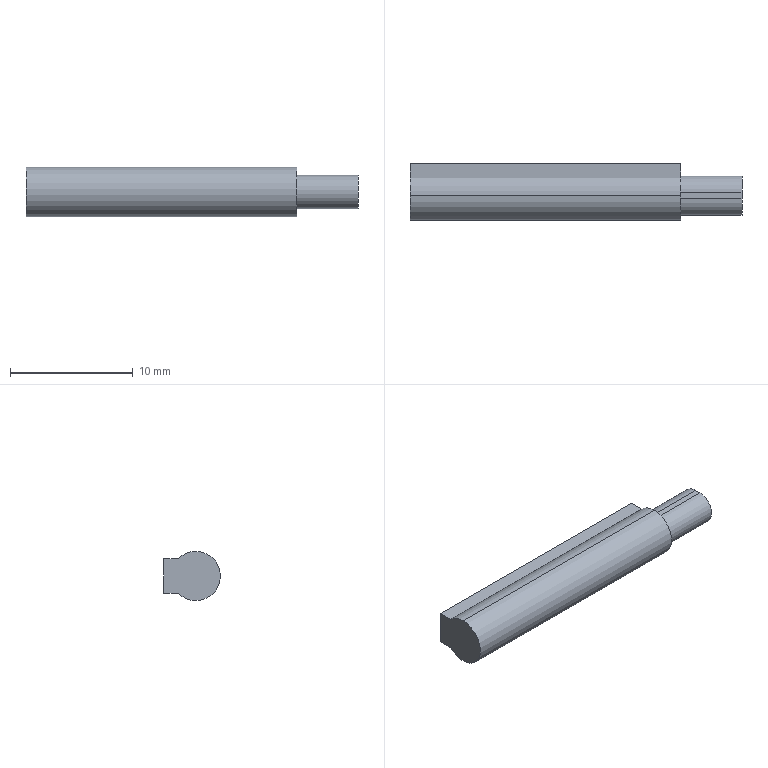Part | SolidWorks | features BaseBody 1 | 1 solid | 16 faces | box 27 x 4.6 x 4 mm | volume 359.458 mm3 | plane 9 | cylinder 7 | commonest cylinder face diameters 4 x3 2 x2 2.7 x2
STEP:
#1=CARTESIAN_POINT('',(22.,1.428,-1.4));
#2=VERTEX_POINT('',#1);
#3=CARTESIAN_POINT('',(22.,0.,-2.));
#4=VERTEX_POINT('',#3);
#5=CARTESIAN_POINT('',(22.,0.,0.));
#6=DIRECTION('',(-1.,0.,0.));
#7=DIRECTION('',(0.,0.,1.));
#8=AXIS2_PLACEMENT_3D('',#5,#6,#7);
#9=CIRCLE('',#8,2.);
#10=EDGE_CURVE('',#2,#4,#9,.T.);
#11=ORIENTED_EDGE('',*,*,#10,.T.);
#12=CARTESIAN_POINT('',(0.,0.,-2.));
#13=VERTEX_POINT('',#12);
#14=CARTESIAN_POINT('',(22.,0.,-2.));
#15=DIRECTION('',(-1.,0.,0.));
#16=VECTOR('',#15,1000.);
#17=LINE('',#14,#16);
#18=EDGE_CURVE('',#4,#13,#17,.T.);
#19=ORIENTED_EDGE('',*,*,#18,.T.);
#20=CARTESIAN_POINT('',(0.,1.428,-1.4));
#21=VERTEX_POINT('',#20);
#22=CARTESIAN_POINT('',(0.,0.,0.));
#23=DIRECTION('',(1.,0.,0.));
#24=DIRECTION('',(0.,0.,1.));
#25=AXIS2_PLACEMENT_3D('',#22,#23,#24);
#26=CIRCLE('',#25,2.);
#27=EDGE_CURVE('',#13,#21,#26,.T.);
#28=ORIENTED_EDGE('',*,*,#27,.T.);
#29=CARTESIAN_POINT('',(22.,1.428,-1.4));
#30=DIRECTION('',(1.,0.,0.));
#31=VECTOR('',#30,1000.);
#32=LINE('',#29,#31);
#33=EDGE_CURVE('',#21,#2,#32,.T.);
#34=ORIENTED_EDGE('',*,*,#33,.T.);
#35=EDGE_LOOP('',(#11,#19,#28,#34));
#36=FACE_OUTER_BOUND('',#35,.T.);
#37=CARTESIAN_POINT('',(22.,0.,0.));
#38=DIRECTION('',(-1.,0.,0.));
#39=DIRECTION('',(0.,0.,1.));
#40=AXIS2_PLACEMENT_3D('',#37,#38,#39);
#41=CYLINDRICAL_SURFACE('',#40,2.);
#42=ADVANCED_FACE('',(#36),#41,.T.);
#43=ORIENTED_EDGE('',*,*,#18,.F.);
#44=CARTESIAN_POINT('',(22.,0.,2.));
#45=VERTEX_POINT('',#44);
#46=CARTESIAN_POINT('',(22.,0.,0.));
#47=DIRECTION('',(-1.,0.,0.));
#48=DIRECTION('',(0.,0.,1.));
#49=AXIS2_PLACEMENT_3D('',#46,#47,#48);
#50=CIRCLE('',#49,2.);
#51=EDGE_CURVE('',#4,#45,#50,.T.);
#52=ORIENTED_EDGE('',*,*,#51,.T.);
#53=CARTESIAN_POINT('',(0.,0.,2.));
#54=VERTEX_POINT('',#53);
#55=CARTESIAN_POINT('',(22.,0.,2.));
#56=DIRECTION('',(-1.,0.,0.));
#57=VECTOR('',#56,1000.);
#58=LINE('',#55,#57);
#59=EDGE_CURVE('',#45,#54,#58,.T.);
#60=ORIENTED_EDGE('',*,*,#59,.T.);
#61=CARTESIAN_POINT('',(0.,0.,0.));
#62=DIRECTION('',(1.,0.,0.));
#63=DIRECTION('',(0.,0.,1.));
#64=AXIS2_PLACEMENT_3D('',#61,#62,#63);
#65=CIRCLE('',#64,2.);
#66=EDGE_CURVE('',#54,#13,#65,.T.);
#67=ORIENTED_EDGE('',*,*,#66,.T.);
#68=EDGE_LOOP('',(#43,#52,#60,#67));
#69=FACE_OUTER_BOUND('',#68,.T.);
#70=CARTESIAN_POINT('',(22.,0.,0.));
#71=DIRECTION('',(-1.,0.,0.));
#72=DIRECTION('',(0.,0.,1.));
#73=AXIS2_PLACEMENT_3D('',#70,#71,#72);
#74=CYLINDRICAL_SURFACE('',#73,2.);
#75=ADVANCED_FACE('',(#69),#74,.T.);
#76=CARTESIAN_POINT('',(2.,2.5,-1.));
#77=VERTEX_POINT('',#76);
#78=CARTESIAN_POINT('',(2.,2.5,1.));
#79=VERTEX_POINT('',#78);
#80=CARTESIAN_POINT('',(2.,2.5,0.));
#81=DIRECTION('',(0.,1.,0.));
#82=DIRECTION('',(0.,0.,1.));
#83=AXIS2_PLACEMENT_3D('',#80,#81,#82);
#84=CIRCLE('',#83,1.);
#85=EDGE_CURVE('',#77,#79,#84,.T.);
#86=ORIENTED_EDGE('',*,*,#85,.F.);
#87=CARTESIAN_POINT('',(2.,2.6,-1.));
#88=VERTEX_POINT('',#87);
#89=CARTESIAN_POINT('',(2.,2.6,-1.));
#90=DIRECTION('',(0.,1.,0.));
#91=VECTOR('',#90,1000.);
#92=LINE('',#89,#91);
#93=EDGE_CURVE('',#77,#88,#92,.T.);
#94=ORIENTED_EDGE('',*,*,#93,.T.);
#95=CARTESIAN_POINT('',(2.,2.6,1.));
#96=VERTEX_POINT('',#95);
#97=CARTESIAN_POINT('',(2.,2.6,0.));
#98=DIRECTION('',(0.,1.,0.));
#99=DIRECTION('',(0.,0.,1.));
#100=AXIS2_PLACEMENT_3D('',#97,#98,#99);
#101=CIRCLE('',#100,1.);
#102=EDGE_CURVE('',#88,#96,#101,.T.);
#103=ORIENTED_EDGE('',*,*,#102,.T.);
#104=CARTESIAN_POINT('',(2.,2.6,1.));
#105=DIRECTION('',(0.,1.,0.));
#106=VECTOR('',#105,1000.);
#107=LINE('',#104,#106);
#108=EDGE_CURVE('',#79,#96,#107,.T.);
#109=ORIENTED_EDGE('',*,*,#108,.F.);
#110=EDGE_LOOP('',(#86,#94,#103,#109));
#111=FACE_OUTER_BOUND('',#110,.T.);
#112=CARTESIAN_POINT('',(2.,2.6,0.));
#113=DIRECTION('',(0.,1.,0.));
#114=DIRECTION('',(0.,0.,1.));
#115=AXIS2_PLACEMENT_3D('',#112,#113,#114);
#116=CYLINDRICAL_SURFACE('',#115,1.);
#117=ADVANCED_FACE('',(#111),#116,.F.);
#118=ORIENTED_EDGE('',*,*,#59,.F.);
#119=CARTESIAN_POINT('',(22.,1.428,1.4));
#120=VERTEX_POINT('',#119);
#121=CARTESIAN_POINT('',(22.,0.,0.));
#122=DIRECTION('',(-1.,0.,0.));
#123=DIRECTION('',(0.,0.,1.));
#124=AXIS2_PLACEMENT_3D('',#121,#122,#123);
#125=CIRCLE('',#124,2.);
#126=EDGE_CURVE('',#45,#120,#125,.T.);
#127=ORIENTED_EDGE('',*,*,#126,.T.);
#128=CARTESIAN_POINT('',(0.,1.428,1.4));
#129=VERTEX_POINT('',#128);
#130=CARTESIAN_POINT('',(22.,1.428,1.4));
#131=DIRECTION('',(-1.,0.,0.));
#132=VECTOR('',#131,1000.);
#133=LINE('',#130,#132);
#134=EDGE_CURVE('',#120,#129,#133,.T.);
#135=ORIENTED_EDGE('',*,*,#134,.T.);
#136=CARTESIAN_POINT('',(0.,0.,0.));
#137=DIRECTION('',(1.,0.,0.));
#138=DIRECTION('',(0.,0.,1.));
#139=AXIS2_PLACEMENT_3D('',#136,#137,#138);
#140=CIRCLE('',#139,2.);
#141=EDGE_CURVE('',#129,#54,#140,.T.);
#142=ORIENTED_EDGE('',*,*,#141,.T.);
#143=EDGE_LOOP('',(#118,#127,#135,#142));
#144=FACE_OUTER_BOUND('',#143,.T.);
#145=CARTESIAN_POINT('',(22.,0.,0.));
#146=DIRECTION('',(-1.,0.,0.));
#147=DIRECTION('',(0.,0.,1.));
#148=AXIS2_PLACEMENT_3D('',#145,#146,#147);
#149=CYLINDRICAL_SURFACE('',#148,2.);
#150=ADVANCED_FACE('',(#144),#149,.T.);
#151=CARTESIAN_POINT('',(0.,2.6,1.4));
#152=VERTEX_POINT('',#151);
#153=CARTESIAN_POINT('',(0.,2.6,1.4));
#154=DIRECTION('',(0.,1.,0.));
#155=VECTOR('',#154,1000.);
#156=LINE('',#153,#155);
#157=EDGE_CURVE('',#129,#152,#156,.T.);
#158=ORIENTED_EDGE('',*,*,#157,.T.);
#159=CARTESIAN_POINT('',(0.,2.6,-1.4));
#160=VERTEX_POINT('',#159);
#161=CARTESIAN_POINT('',(0.,2.6,0.));
#162=DIRECTION('',(0.,0.,1.));
#163=VECTOR('',#162,1000.);
#164=LINE('',#161,#163);
#165=EDGE_CURVE('',#160,#152,#164,.T.);
#166=ORIENTED_EDGE('',*,*,#165,.F.);
#167=CARTESIAN_POINT('',(0.,1.428,-1.4));
#168=DIRECTION('',(0.,-1.,0.));
#169=VECTOR('',#168,1000.);
#170=LINE('',#167,#169);
#171=EDGE_CURVE('',#160,#21,#170,.T.);
#172=ORIENTED_EDGE('',*,*,#171,.T.);
#173=ORIENTED_EDGE('',*,*,#27,.F.);
#174=ORIENTED_EDGE('',*,*,#66,.F.);
#175=ORIENTED_EDGE('',*,*,#141,.F.);
#176=EDGE_LOOP('',(#158,#166,#172,#173,#174,#175));
#177=FACE_OUTER_BOUND('',#176,.T.);
#178=CARTESIAN_POINT('',(0.,0.,0.));
#179=DIRECTION('',(1.,0.,0.));
#180=DIRECTION('',(0.,0.,-1.));
#181=AXIS2_PLACEMENT_3D('',#178,#179,#180);
#182=PLANE('',#181);
#183=ADVANCED_FACE('',(#177),#182,.F.);
#184=CARTESIAN_POINT('',(22.,-0.25,1.35));
#185=VERTEX_POINT('',#184);
#186=CARTESIAN_POINT('',(22.,0.25,1.35));
#187=VERTEX_POINT('',#186);
#188=CARTESIAN_POINT('',(22.,0.25,1.35));
#189=DIRECTION('',(0.,1.,0.));
#190=VECTOR('',#189,1000.);
#191=LINE('',#188,#190);
#192=EDGE_CURVE('',#185,#187,#191,.T.);
#193=ORIENTED_EDGE('',*,*,#192,.T.);
#194=CARTESIAN_POINT('',(22.,0.25,-1.35));
#195=VERTEX_POINT('',#194);
#196=CARTESIAN_POINT('',(22.,0.25,0.));
#197=DIRECTION('',(-1.,0.,0.));
#198=DIRECTION('',(0.,0.,1.));
#199=AXIS2_PLACEMENT_3D('',#196,#197,#198);
#200=CIRCLE('',#199,1.35);
#201=EDGE_CURVE('',#187,#195,#200,.T.);
#202=ORIENTED_EDGE('',*,*,#201,.T.);
#203=CARTESIAN_POINT('',(22.,-0.25,-1.35));
#204=VERTEX_POINT('',#203);
#205=CARTESIAN_POINT('',(22.,-0.25,-1.35));
#206=DIRECTION('',(0.,-1.,0.));
#207=VECTOR('',#206,1000.);
#208=LINE('',#205,#207);
#209=EDGE_CURVE('',#195,#204,#208,.T.);
#210=ORIENTED_EDGE('',*,*,#209,.T.);
#211=CARTESIAN_POINT('',(22.,-0.25,0.));
#212=DIRECTION('',(-1.,0.,0.));
#213=DIRECTION('',(0.,0.,1.));
#214=AXIS2_PLACEMENT_3D('',#211,#212,#213);
#215=CIRCLE('',#214,1.35);
#216=EDGE_CURVE('',#204,#185,#215,.T.);
#217=ORIENTED_EDGE('',*,*,#216,.T.);
#218=EDGE_LOOP('',(#193,#202,#210,#217));
#219=FACE_BOUND('',#218,.T.);
#220=CARTESIAN_POINT('',(22.,2.6,-1.4));
#221=VERTEX_POINT('',#220);
#222=CARTESIAN_POINT('',(22.,2.6,1.4));
#223=VERTEX_POINT('',#222);
#224=CARTESIAN_POINT('',(22.,2.6,0.));
#225=DIRECTION('',(0.,0.,1.));
#226=VECTOR('',#225,1000.);
#227=LINE('',#224,#226);
#228=EDGE_CURVE('',#221,#223,#227,.T.);
#229=ORIENTED_EDGE('',*,*,#228,.T.);
#230=CARTESIAN_POINT('',(22.,0.,1.4));
#231=DIRECTION('',(0.,-1.,0.));
#232=VECTOR('',#231,1000.);
#233=LINE('',#230,#232);
#234=EDGE_CURVE('',#223,#120,#233,.T.);
#235=ORIENTED_EDGE('',*,*,#234,.T.);
#236=ORIENTED_EDGE('',*,*,#126,.F.);
#237=ORIENTED_EDGE('',*,*,#51,.F.);
#238=ORIENTED_EDGE('',*,*,#10,.F.);
#239=CARTESIAN_POINT('',(22.,1.428,-1.4));
#240=DIRECTION('',(0.,1.,0.));
#241=VECTOR('',#240,1000.);
#242=LINE('',#239,#241);
#243=EDGE_CURVE('',#2,#221,#242,.T.);
#244=ORIENTED_EDGE('',*,*,#243,.T.);
#245=EDGE_LOOP('',(#229,#235,#236,#237,#238,#244));
#246=FACE_OUTER_BOUND('',#245,.T.);
#247=CARTESIAN_POINT('',(22.,0.,0.));
#248=DIRECTION('',(1.,0.,0.));
#249=DIRECTION('',(0.,0.,-1.));
#250=AXIS2_PLACEMENT_3D('',#247,#248,#249);
#251=PLANE('',#250);
#252=ADVANCED_FACE('',(#219,#246),#251,.T.);
#253=CARTESIAN_POINT('',(22.,2.6,1.4));
#254=DIRECTION('',(-1.,0.,0.));
#255=VECTOR('',#254,1000.);
#256=LINE('',#253,#255);
#257=EDGE_CURVE('',#223,#152,#256,.T.);
#258=ORIENTED_EDGE('',*,*,#257,.F.);
#259=ORIENTED_EDGE('',*,*,#228,.F.);
#260=CARTESIAN_POINT('',(22.,2.6,-1.4));
#261=DIRECTION('',(1.,0.,0.));
#262=VECTOR('',#261,1000.);
#263=LINE('',#260,#262);
#264=EDGE_CURVE('',#160,#221,#263,.T.);
#265=ORIENTED_EDGE('',*,*,#264,.F.);
#266=ORIENTED_EDGE('',*,*,#165,.T.);
#267=EDGE_LOOP('',(#258,#259,#265,#266));
#268=FACE_OUTER_BOUND('',#267,.T.);
#269=CARTESIAN_POINT('',(2.,2.6,0.));
#270=DIRECTION('',(0.,1.,0.));
#271=DIRECTION('',(0.,0.,1.));
#272=AXIS2_PLACEMENT_3D('',#269,#270,#271);
#273=CIRCLE('',#272,1.);
#274=EDGE_CURVE('',#96,#88,#273,.T.);
#275=ORIENTED_EDGE('',*,*,#274,.F.);
#276=ORIENTED_EDGE('',*,*,#102,.F.);
#277=EDGE_LOOP('',(#275,#276));
#278=FACE_BOUND('',#277,.T.);
#279=CARTESIAN_POINT('',(22.,2.6,-1.4));
#280=DIRECTION('',(0.,-1.,0.));
#281=DIRECTION('',(0.,0.,-1.));
#282=AXIS2_PLACEMENT_3D('',#279,#280,#281);
#283=PLANE('',#282);
#284=ADVANCED_FACE('',(#268,#278),#283,.F.);
#285=ORIENTED_EDGE('',*,*,#134,.F.);
#286=ORIENTED_EDGE('',*,*,#234,.F.);
#287=ORIENTED_EDGE('',*,*,#257,.T.);
#288=ORIENTED_EDGE('',*,*,#157,.F.);
#289=EDGE_LOOP('',(#285,#286,#287,#288));
#290=FACE_OUTER_BOUND('',#289,.T.);
#291=CARTESIAN_POINT('',(22.,2.6,1.4));
#292=DIRECTION('',(0.,0.,-1.));
#293=DIRECTION('',(-1.,0.,0.));
#294=AXIS2_PLACEMENT_3D('',#291,#292,#293);
#295=PLANE('',#294);
#296=ADVANCED_FACE('',(#290),#295,.F.);
#297=CARTESIAN_POINT('',(27.,0.25,1.35));
#298=VERTEX_POINT('',#297);
#299=CARTESIAN_POINT('',(27.,0.25,-1.35));
#300=VERTEX_POINT('',#299);
#301=CARTESIAN_POINT('',(27.,0.25,0.));
#302=DIRECTION('',(-1.,0.,0.));
#303=DIRECTION('',(0.,0.,1.));
#304=AXIS2_PLACEMENT_3D('',#301,#302,#303);
#305=CIRCLE('',#304,1.35);
#306=EDGE_CURVE('',#298,#300,#305,.T.);
#307=ORIENTED_EDGE('',*,*,#306,.T.);
#308=CARTESIAN_POINT('',(27.,0.25,-1.35));
#309=DIRECTION('',(-1.,0.,0.));
#310=VECTOR('',#309,1000.);
#311=LINE('',#308,#310);
#312=EDGE_CURVE('',#300,#195,#311,.T.);
#313=ORIENTED_EDGE('',*,*,#312,.T.);
#314=ORIENTED_EDGE('',*,*,#201,.F.);
#315=CARTESIAN_POINT('',(27.,0.25,1.35));
#316=DIRECTION('',(1.,0.,0.));
#317=VECTOR('',#316,1000.);
#318=LINE('',#315,#317);
#319=EDGE_CURVE('',#187,#298,#318,.T.);
#320=ORIENTED_EDGE('',*,*,#319,.T.);
#321=EDGE_LOOP('',(#307,#313,#314,#320));
#322=FACE_OUTER_BOUND('',#321,.T.);
#323=CARTESIAN_POINT('',(27.,0.25,0.));
#324=DIRECTION('',(-1.,0.,0.));
#325=DIRECTION('',(0.,0.,1.));
#326=AXIS2_PLACEMENT_3D('',#323,#324,#325);
#327=CYLINDRICAL_SURFACE('',#326,1.35);
#328=ADVANCED_FACE('',(#322),#327,.T.);
#329=CARTESIAN_POINT('',(27.,-0.25,-1.35));
#330=VERTEX_POINT('',#329);
#331=CARTESIAN_POINT('',(27.,-0.25,1.35));
#332=VERTEX_POINT('',#331);
#333=CARTESIAN_POINT('',(27.,-0.25,0.));
#334=DIRECTION('',(-1.,0.,0.));
#335=DIRECTION('',(0.,0.,1.));
#336=AXIS2_PLACEMENT_3D('',#333,#334,#335);
#337=CIRCLE('',#336,1.35);
#338=EDGE_CURVE('',#330,#332,#337,.T.);
#339=ORIENTED_EDGE('',*,*,#338,.T.);
#340=CARTESIAN_POINT('',(27.,-0.25,1.35));
#341=DIRECTION('',(-1.,0.,0.));
#342=VECTOR('',#341,1000.);
#343=LINE('',#340,#342);
#344=EDGE_CURVE('',#332,#185,#343,.T.);
#345=ORIENTED_EDGE('',*,*,#344,.T.);
#346=ORIENTED_EDGE('',*,*,#216,.F.);
#347=CARTESIAN_POINT('',(27.,-0.25,-1.35));
#348=DIRECTION('',(1.,0.,0.));
#349=VECTOR('',#348,1000.);
#350=LINE('',#347,#349);
#351=EDGE_CURVE('',#204,#330,#350,.T.);
#352=ORIENTED_EDGE('',*,*,#351,.T.);
#353=EDGE_LOOP('',(#339,#345,#346,#352));
#354=FACE_OUTER_BOUND('',#353,.T.);
#355=CARTESIAN_POINT('',(27.,-0.25,0.));
#356=DIRECTION('',(-1.,0.,0.));
#357=DIRECTION('',(0.,0.,1.));
#358=AXIS2_PLACEMENT_3D('',#355,#356,#357);
#359=CYLINDRICAL_SURFACE('',#358,1.35);
#360=ADVANCED_FACE('',(#354),#359,.T.);
#361=ORIENTED_EDGE('',*,*,#264,.T.);
#362=ORIENTED_EDGE('',*,*,#243,.F.);
#363=ORIENTED_EDGE('',*,*,#33,.F.);
#364=ORIENTED_EDGE('',*,*,#171,.F.);
#365=EDGE_LOOP('',(#361,#362,#363,#364));
#366=FACE_OUTER_BOUND('',#365,.T.);
#367=CARTESIAN_POINT('',(22.,1.428,-1.4));
#368=DIRECTION('',(0.,0.,1.));
#369=DIRECTION('',(1.,0.,0.));
#370=AXIS2_PLACEMENT_3D('',#367,#368,#369);
#371=PLANE('',#370);
#372=ADVANCED_FACE('',(#366),#371,.F.);
#373=ORIENTED_EDGE('',*,*,#93,.F.);
#374=CARTESIAN_POINT('',(2.,2.5,0.));
#375=DIRECTION('',(0.,1.,0.));
#376=DIRECTION('',(0.,0.,1.));
#377=AXIS2_PLACEMENT_3D('',#374,#375,#376);
#378=CIRCLE('',#377,1.);
#379=EDGE_CURVE('',#79,#77,#378,.T.);
#380=ORIENTED_EDGE('',*,*,#379,.F.);
#381=ORIENTED_EDGE('',*,*,#108,.T.);
#382=ORIENTED_EDGE('',*,*,#274,.T.);
#383=EDGE_LOOP('',(#373,#380,#381,#382));
#384=FACE_OUTER_BOUND('',#383,.T.);
#385=CARTESIAN_POINT('',(2.,2.6,0.));
#386=DIRECTION('',(0.,1.,0.));
#387=DIRECTION('',(0.,0.,1.));
#388=AXIS2_PLACEMENT_3D('',#385,#386,#387);
#389=CYLINDRICAL_SURFACE('',#388,1.);
#390=ADVANCED_FACE('',(#384),#389,.F.);
#391=ORIENTED_EDGE('',*,*,#312,.F.);
#392=CARTESIAN_POINT('',(27.,-0.25,-1.35));
#393=DIRECTION('',(0.,1.,0.));
#394=VECTOR('',#393,1000.);
#395=LINE('',#392,#394);
#396=EDGE_CURVE('',#330,#300,#395,.T.);
#397=ORIENTED_EDGE('',*,*,#396,.F.);
#398=ORIENTED_EDGE('',*,*,#351,.F.);
#399=ORIENTED_EDGE('',*,*,#209,.F.);
#400=EDGE_LOOP('',(#391,#397,#398,#399));
#401=FACE_OUTER_BOUND('',#400,.T.);
#402=CARTESIAN_POINT('',(27.,-0.25,-1.35));
#403=DIRECTION('',(0.,0.,1.));
#404=DIRECTION('',(1.,0.,0.));
#405=AXIS2_PLACEMENT_3D('',#402,#403,#404);
#406=PLANE('',#405);
#407=ADVANCED_FACE('',(#401),#406,.F.);
#408=ORIENTED_EDGE('',*,*,#306,.F.);
#409=CARTESIAN_POINT('',(27.,-0.25,1.35));
#410=DIRECTION('',(0.,-1.,0.));
#411=VECTOR('',#410,1000.);
#412=LINE('',#409,#411);
#413=EDGE_CURVE('',#298,#332,#412,.T.);
#414=ORIENTED_EDGE('',*,*,#413,.T.);
#415=ORIENTED_EDGE('',*,*,#338,.F.);
#416=ORIENTED_EDGE('',*,*,#396,.T.);
#417=EDGE_LOOP('',(#408,#414,#415,#416));
#418=FACE_OUTER_BOUND('',#417,.T.);
#419=CARTESIAN_POINT('',(27.,-0.25,0.));
#420=DIRECTION('',(1.,0.,0.));
#421=DIRECTION('',(0.,0.,-1.));
#422=AXIS2_PLACEMENT_3D('',#419,#420,#421);
#423=PLANE('',#422);
#424=ADVANCED_FACE('',(#418),#423,.T.);
#425=ORIENTED_EDGE('',*,*,#344,.F.);
#426=ORIENTED_EDGE('',*,*,#413,.F.);
#427=ORIENTED_EDGE('',*,*,#319,.F.);
#428=ORIENTED_EDGE('',*,*,#192,.F.);
#429=EDGE_LOOP('',(#425,#426,#427,#428));
#430=FACE_OUTER_BOUND('',#429,.T.);
#431=CARTESIAN_POINT('',(27.,0.25,1.35));
#432=DIRECTION('',(0.,0.,-1.));
#433=DIRECTION('',(-1.,0.,0.));
#434=AXIS2_PLACEMENT_3D('',#431,#432,#433);
#435=PLANE('',#434);
#436=ADVANCED_FACE('',(#430),#435,.F.);
#437=ORIENTED_EDGE('',*,*,#379,.T.);
#438=ORIENTED_EDGE('',*,*,#85,.T.);
#439=EDGE_LOOP('',(#437,#438));
#440=FACE_OUTER_BOUND('',#439,.T.);
#441=CARTESIAN_POINT('',(2.,2.5,0.));
#442=DIRECTION('',(0.,-1.,0.));
#443=DIRECTION('',(0.,0.,-1.));
#444=AXIS2_PLACEMENT_3D('',#441,#442,#443);
#445=PLANE('',#444);
#446=ADVANCED_FACE('',(#440),#445,.F.);
#447=CLOSED_SHELL('',(#42,#75,#117,#150,#183,#252,#284,#296,#328,#360,#372,#390,#407,#424,#436,#446));
#448=MANIFOLD_SOLID_BREP('',#447);
#449=CARTESIAN_POINT('',(0.,0.,0.));
#450=DIRECTION('',(0.,0.,1.));
#451=DIRECTION('',(1.,0.,0.));
#452=AXIS2_PLACEMENT_3D('',#449,#450,#451);
#453=(LENGTH_UNIT()NAMED_UNIT(*)SI_UNIT(.MILLI.,.METRE.));
#454=UNCERTAINTY_MEASURE_WITH_UNIT(LENGTH_MEASURE(0.00001),#453,'','');
#455=(NAMED_UNIT(*)PLANE_ANGLE_UNIT()SI_UNIT($,.RADIAN.));
#456=(NAMED_UNIT(*)SI_UNIT($,.STERADIAN.)SOLID_ANGLE_UNIT());
#457=(GEOMETRIC_REPRESENTATION_CONTEXT(3)GLOBAL_UNCERTAINTY_ASSIGNED_CONTEXT((#454))GLOBAL_UNIT_ASSIGNED_CONTEXT((#453,#455,#456))REPRESENTATION_CONTEXT('',''));
#458=ADVANCED_BREP_SHAPE_REPRESENTATION('',(#448,#452),#457);